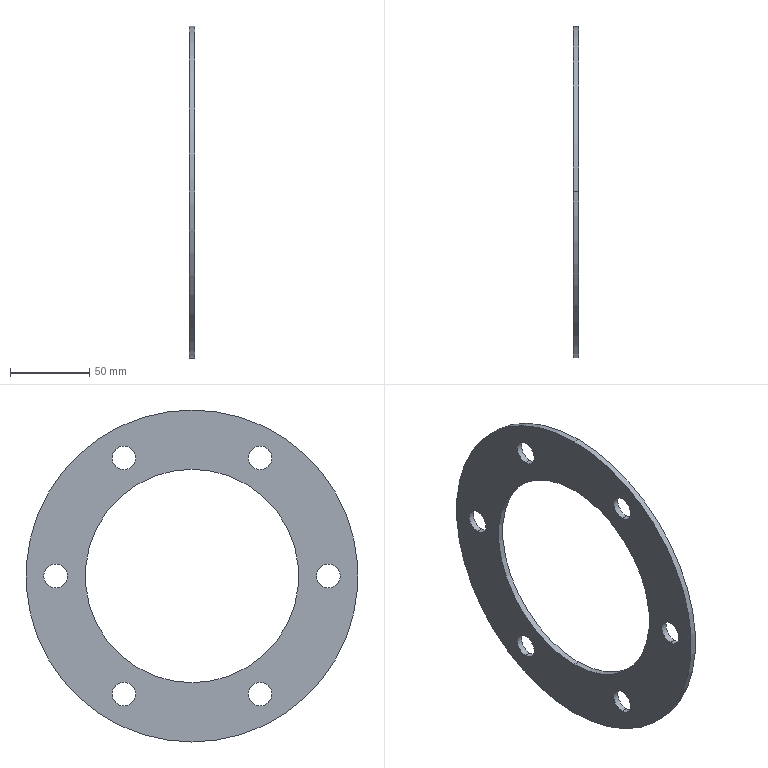Part | SolidWorks | features ICE 1, Revolution 1, Scale 1 | 1 solid | 18 faces | box 3.75 x 210 x 210 mm | volume 72232 mm3 | cylinder 16 | plane 2 | commonest cylinder face diameters 15 x12 135 x2 210 x2
STEP:
#1=CARTESIAN_POINT('',(-0.875,-43.125,67.195));
#2=VERTEX_POINT('',#1);
#3=CARTESIAN_POINT('',(-0.875,-43.125,82.195));
#4=VERTEX_POINT('',#3);
#5=CARTESIAN_POINT('',(-0.875,-43.125,74.695));
#6=DIRECTION('',(-1.,0.,0.));
#7=DIRECTION('',(0.,0.,-1.));
#8=AXIS2_PLACEMENT_3D('',#5,#6,#7);
#9=CIRCLE('',#8,7.5);
#10=EDGE_CURVE('',#2,#4,#9,.T.);
#11=ORIENTED_EDGE('',*,*,#10,.T.);
#12=CARTESIAN_POINT('',(2.875,-43.125,82.195));
#13=VERTEX_POINT('',#12);
#14=CARTESIAN_POINT('',(-15.875,-43.125,82.195));
#15=DIRECTION('',(1.,0.,0.));
#16=VECTOR('',#15,1000.);
#17=LINE('',#14,#16);
#18=EDGE_CURVE('',#4,#13,#17,.T.);
#19=ORIENTED_EDGE('',*,*,#18,.T.);
#20=CARTESIAN_POINT('',(2.875,-43.125,67.195));
#21=VERTEX_POINT('',#20);
#22=CARTESIAN_POINT('',(2.875,-43.125,74.695));
#23=DIRECTION('',(-1.,0.,0.));
#24=DIRECTION('',(0.,0.,1.));
#25=AXIS2_PLACEMENT_3D('',#22,#23,#24);
#26=CIRCLE('',#25,7.5);
#27=EDGE_CURVE('',#21,#13,#26,.T.);
#28=ORIENTED_EDGE('',*,*,#27,.F.);
#29=CARTESIAN_POINT('',(-15.875,-43.125,67.195));
#30=DIRECTION('',(1.,0.,0.));
#31=VECTOR('',#30,1000.);
#32=LINE('',#29,#31);
#33=EDGE_CURVE('',#2,#21,#32,.T.);
#34=ORIENTED_EDGE('',*,*,#33,.F.);
#35=EDGE_LOOP('',(#11,#19,#28,#34));
#36=FACE_OUTER_BOUND('',#35,.T.);
#37=CARTESIAN_POINT('',(-15.875,-43.125,74.695));
#38=DIRECTION('',(1.,0.,0.));
#39=DIRECTION('',(0.,0.,-1.));
#40=AXIS2_PLACEMENT_3D('',#37,#38,#39);
#41=CYLINDRICAL_SURFACE('',#40,7.5);
#42=ADVANCED_FACE('',(#36),#41,.F.);
#43=CARTESIAN_POINT('',(-0.875,-86.25,-7.5));
#44=VERTEX_POINT('',#43);
#45=CARTESIAN_POINT('',(-0.875,-86.25,7.5));
#46=VERTEX_POINT('',#45);
#47=CARTESIAN_POINT('',(-0.875,-86.25,0.));
#48=DIRECTION('',(-1.,0.,0.));
#49=DIRECTION('',(0.,0.,-1.));
#50=AXIS2_PLACEMENT_3D('',#47,#48,#49);
#51=CIRCLE('',#50,7.5);
#52=EDGE_CURVE('',#44,#46,#51,.T.);
#53=ORIENTED_EDGE('',*,*,#52,.T.);
#54=CARTESIAN_POINT('',(2.875,-86.25,7.5));
#55=VERTEX_POINT('',#54);
#56=CARTESIAN_POINT('',(-15.875,-86.25,7.5));
#57=DIRECTION('',(1.,0.,0.));
#58=VECTOR('',#57,1000.);
#59=LINE('',#56,#58);
#60=EDGE_CURVE('',#46,#55,#59,.T.);
#61=ORIENTED_EDGE('',*,*,#60,.T.);
#62=CARTESIAN_POINT('',(2.875,-86.25,-7.5));
#63=VERTEX_POINT('',#62);
#64=CARTESIAN_POINT('',(2.875,-86.25,0.));
#65=DIRECTION('',(-1.,0.,0.));
#66=DIRECTION('',(0.,0.,1.));
#67=AXIS2_PLACEMENT_3D('',#64,#65,#66);
#68=CIRCLE('',#67,7.5);
#69=EDGE_CURVE('',#63,#55,#68,.T.);
#70=ORIENTED_EDGE('',*,*,#69,.F.);
#71=CARTESIAN_POINT('',(-15.875,-86.25,-7.5));
#72=DIRECTION('',(1.,0.,0.));
#73=VECTOR('',#72,1000.);
#74=LINE('',#71,#73);
#75=EDGE_CURVE('',#44,#63,#74,.T.);
#76=ORIENTED_EDGE('',*,*,#75,.F.);
#77=EDGE_LOOP('',(#53,#61,#70,#76));
#78=FACE_OUTER_BOUND('',#77,.T.);
#79=CARTESIAN_POINT('',(-15.875,-86.25,0.));
#80=DIRECTION('',(1.,0.,0.));
#81=DIRECTION('',(0.,0.,-1.));
#82=AXIS2_PLACEMENT_3D('',#79,#80,#81);
#83=CYLINDRICAL_SURFACE('',#82,7.5);
#84=ADVANCED_FACE('',(#78),#83,.F.);
#85=CARTESIAN_POINT('',(-0.875,-43.125,-82.195));
#86=VERTEX_POINT('',#85);
#87=CARTESIAN_POINT('',(-0.875,-43.125,-67.195));
#88=VERTEX_POINT('',#87);
#89=CARTESIAN_POINT('',(-0.875,-43.125,-74.695));
#90=DIRECTION('',(-1.,0.,0.));
#91=DIRECTION('',(0.,0.,-1.));
#92=AXIS2_PLACEMENT_3D('',#89,#90,#91);
#93=CIRCLE('',#92,7.5);
#94=EDGE_CURVE('',#86,#88,#93,.T.);
#95=ORIENTED_EDGE('',*,*,#94,.T.);
#96=CARTESIAN_POINT('',(2.875,-43.125,-67.195));
#97=VERTEX_POINT('',#96);
#98=CARTESIAN_POINT('',(-15.875,-43.125,-67.195));
#99=DIRECTION('',(1.,0.,0.));
#100=VECTOR('',#99,1000.);
#101=LINE('',#98,#100);
#102=EDGE_CURVE('',#88,#97,#101,.T.);
#103=ORIENTED_EDGE('',*,*,#102,.T.);
#104=CARTESIAN_POINT('',(2.875,-43.125,-82.195));
#105=VERTEX_POINT('',#104);
#106=CARTESIAN_POINT('',(2.875,-43.125,-74.695));
#107=DIRECTION('',(-1.,0.,0.));
#108=DIRECTION('',(0.,0.,1.));
#109=AXIS2_PLACEMENT_3D('',#106,#107,#108);
#110=CIRCLE('',#109,7.5);
#111=EDGE_CURVE('',#105,#97,#110,.T.);
#112=ORIENTED_EDGE('',*,*,#111,.F.);
#113=CARTESIAN_POINT('',(-15.875,-43.125,-82.195));
#114=DIRECTION('',(1.,0.,0.));
#115=VECTOR('',#114,1000.);
#116=LINE('',#113,#115);
#117=EDGE_CURVE('',#86,#105,#116,.T.);
#118=ORIENTED_EDGE('',*,*,#117,.F.);
#119=EDGE_LOOP('',(#95,#103,#112,#118));
#120=FACE_OUTER_BOUND('',#119,.T.);
#121=CARTESIAN_POINT('',(-15.875,-43.125,-74.695));
#122=DIRECTION('',(1.,0.,0.));
#123=DIRECTION('',(0.,0.,-1.));
#124=AXIS2_PLACEMENT_3D('',#121,#122,#123);
#125=CYLINDRICAL_SURFACE('',#124,7.5);
#126=ADVANCED_FACE('',(#120),#125,.F.);
#127=CARTESIAN_POINT('',(-0.875,43.125,-67.195));
#128=VERTEX_POINT('',#127);
#129=CARTESIAN_POINT('',(-0.875,43.125,-82.195));
#130=VERTEX_POINT('',#129);
#131=CARTESIAN_POINT('',(-0.875,43.125,-74.695));
#132=DIRECTION('',(1.,0.,0.));
#133=DIRECTION('',(0.,0.,-1.));
#134=AXIS2_PLACEMENT_3D('',#131,#132,#133);
#135=CIRCLE('',#134,7.5);
#136=EDGE_CURVE('',#128,#130,#135,.T.);
#137=ORIENTED_EDGE('',*,*,#136,.F.);
#138=CARTESIAN_POINT('',(2.875,43.125,-67.195));
#139=VERTEX_POINT('',#138);
#140=CARTESIAN_POINT('',(-15.875,43.125,-67.195));
#141=DIRECTION('',(1.,0.,0.));
#142=VECTOR('',#141,1000.);
#143=LINE('',#140,#142);
#144=EDGE_CURVE('',#128,#139,#143,.T.);
#145=ORIENTED_EDGE('',*,*,#144,.T.);
#146=CARTESIAN_POINT('',(2.875,43.125,-82.195));
#147=VERTEX_POINT('',#146);
#148=CARTESIAN_POINT('',(2.875,43.125,-74.695));
#149=DIRECTION('',(1.,0.,0.));
#150=DIRECTION('',(0.,0.,-1.));
#151=AXIS2_PLACEMENT_3D('',#148,#149,#150);
#152=CIRCLE('',#151,7.5);
#153=EDGE_CURVE('',#139,#147,#152,.T.);
#154=ORIENTED_EDGE('',*,*,#153,.T.);
#155=CARTESIAN_POINT('',(-15.875,43.125,-82.195));
#156=DIRECTION('',(1.,0.,0.));
#157=VECTOR('',#156,1000.);
#158=LINE('',#155,#157);
#159=EDGE_CURVE('',#130,#147,#158,.T.);
#160=ORIENTED_EDGE('',*,*,#159,.F.);
#161=EDGE_LOOP('',(#137,#145,#154,#160));
#162=FACE_OUTER_BOUND('',#161,.T.);
#163=CARTESIAN_POINT('',(-15.875,43.125,-74.695));
#164=DIRECTION('',(1.,0.,0.));
#165=DIRECTION('',(0.,0.,-1.));
#166=AXIS2_PLACEMENT_3D('',#163,#164,#165);
#167=CYLINDRICAL_SURFACE('',#166,7.5);
#168=ADVANCED_FACE('',(#162),#167,.F.);
#169=CARTESIAN_POINT('',(-0.875,43.125,82.195));
#170=VERTEX_POINT('',#169);
#171=CARTESIAN_POINT('',(-0.875,43.125,67.195));
#172=VERTEX_POINT('',#171);
#173=CARTESIAN_POINT('',(-0.875,43.125,74.695));
#174=DIRECTION('',(1.,0.,0.));
#175=DIRECTION('',(0.,0.,-1.));
#176=AXIS2_PLACEMENT_3D('',#173,#174,#175);
#177=CIRCLE('',#176,7.5);
#178=EDGE_CURVE('',#170,#172,#177,.T.);
#179=ORIENTED_EDGE('',*,*,#178,.F.);
#180=CARTESIAN_POINT('',(2.875,43.125,82.195));
#181=VERTEX_POINT('',#180);
#182=CARTESIAN_POINT('',(-15.875,43.125,82.195));
#183=DIRECTION('',(1.,0.,0.));
#184=VECTOR('',#183,1000.);
#185=LINE('',#182,#184);
#186=EDGE_CURVE('',#170,#181,#185,.T.);
#187=ORIENTED_EDGE('',*,*,#186,.T.);
#188=CARTESIAN_POINT('',(2.875,43.125,67.195));
#189=VERTEX_POINT('',#188);
#190=CARTESIAN_POINT('',(2.875,43.125,74.695));
#191=DIRECTION('',(1.,0.,0.));
#192=DIRECTION('',(0.,0.,-1.));
#193=AXIS2_PLACEMENT_3D('',#190,#191,#192);
#194=CIRCLE('',#193,7.5);
#195=EDGE_CURVE('',#181,#189,#194,.T.);
#196=ORIENTED_EDGE('',*,*,#195,.T.);
#197=CARTESIAN_POINT('',(-15.875,43.125,67.195));
#198=DIRECTION('',(1.,0.,0.));
#199=VECTOR('',#198,1000.);
#200=LINE('',#197,#199);
#201=EDGE_CURVE('',#172,#189,#200,.T.);
#202=ORIENTED_EDGE('',*,*,#201,.F.);
#203=EDGE_LOOP('',(#179,#187,#196,#202));
#204=FACE_OUTER_BOUND('',#203,.T.);
#205=CARTESIAN_POINT('',(-15.875,43.125,74.695));
#206=DIRECTION('',(1.,0.,0.));
#207=DIRECTION('',(0.,0.,-1.));
#208=AXIS2_PLACEMENT_3D('',#205,#206,#207);
#209=CYLINDRICAL_SURFACE('',#208,7.5);
#210=ADVANCED_FACE('',(#204),#209,.F.);
#211=CARTESIAN_POINT('',(-0.875,86.25,7.5));
#212=VERTEX_POINT('',#211);
#213=CARTESIAN_POINT('',(-0.875,86.25,-7.5));
#214=VERTEX_POINT('',#213);
#215=CARTESIAN_POINT('',(-0.875,86.25,0.));
#216=DIRECTION('',(1.,0.,0.));
#217=DIRECTION('',(0.,0.,-1.));
#218=AXIS2_PLACEMENT_3D('',#215,#216,#217);
#219=CIRCLE('',#218,7.5);
#220=EDGE_CURVE('',#212,#214,#219,.T.);
#221=ORIENTED_EDGE('',*,*,#220,.F.);
#222=CARTESIAN_POINT('',(2.875,86.25,7.5));
#223=VERTEX_POINT('',#222);
#224=CARTESIAN_POINT('',(-15.875,86.25,7.5));
#225=DIRECTION('',(1.,0.,0.));
#226=VECTOR('',#225,1000.);
#227=LINE('',#224,#226);
#228=EDGE_CURVE('',#212,#223,#227,.T.);
#229=ORIENTED_EDGE('',*,*,#228,.T.);
#230=CARTESIAN_POINT('',(2.875,86.25,-7.5));
#231=VERTEX_POINT('',#230);
#232=CARTESIAN_POINT('',(2.875,86.25,0.));
#233=DIRECTION('',(1.,0.,0.));
#234=DIRECTION('',(0.,0.,-1.));
#235=AXIS2_PLACEMENT_3D('',#232,#233,#234);
#236=CIRCLE('',#235,7.5);
#237=EDGE_CURVE('',#223,#231,#236,.T.);
#238=ORIENTED_EDGE('',*,*,#237,.T.);
#239=CARTESIAN_POINT('',(-15.875,86.25,-7.5));
#240=DIRECTION('',(1.,0.,0.));
#241=VECTOR('',#240,1000.);
#242=LINE('',#239,#241);
#243=EDGE_CURVE('',#214,#231,#242,.T.);
#244=ORIENTED_EDGE('',*,*,#243,.F.);
#245=EDGE_LOOP('',(#221,#229,#238,#244));
#246=FACE_OUTER_BOUND('',#245,.T.);
#247=CARTESIAN_POINT('',(-15.875,86.25,0.));
#248=DIRECTION('',(1.,0.,0.));
#249=DIRECTION('',(0.,0.,-1.));
#250=AXIS2_PLACEMENT_3D('',#247,#248,#249);
#251=CYLINDRICAL_SURFACE('',#250,7.5);
#252=ADVANCED_FACE('',(#246),#251,.F.);
#253=CARTESIAN_POINT('',(2.875,0.,105.));
#254=VERTEX_POINT('',#253);
#255=CARTESIAN_POINT('',(2.875,0.,-105.));
#256=VERTEX_POINT('',#255);
#257=CARTESIAN_POINT('',(2.875,0.,0.));
#258=DIRECTION('',(-1.,0.,0.));
#259=DIRECTION('',(0.,0.,1.));
#260=AXIS2_PLACEMENT_3D('',#257,#258,#259);
#261=CIRCLE('',#260,105.);
#262=EDGE_CURVE('',#254,#256,#261,.T.);
#263=ORIENTED_EDGE('',*,*,#262,.T.);
#264=CARTESIAN_POINT('',(-0.875,0.,-105.));
#265=VERTEX_POINT('',#264);
#266=CARTESIAN_POINT('',(-0.875,0.,-105.));
#267=DIRECTION('',(-1.,0.,0.));
#268=VECTOR('',#267,1000.);
#269=LINE('',#266,#268);
#270=EDGE_CURVE('',#256,#265,#269,.T.);
#271=ORIENTED_EDGE('',*,*,#270,.T.);
#272=CARTESIAN_POINT('',(-0.875,0.,105.));
#273=VERTEX_POINT('',#272);
#274=CARTESIAN_POINT('',(-0.875,0.,0.));
#275=DIRECTION('',(-1.,0.,0.));
#276=DIRECTION('',(0.,0.,1.));
#277=AXIS2_PLACEMENT_3D('',#274,#275,#276);
#278=CIRCLE('',#277,105.);
#279=EDGE_CURVE('',#273,#265,#278,.T.);
#280=ORIENTED_EDGE('',*,*,#279,.F.);
#281=CARTESIAN_POINT('',(-0.875,0.,105.));
#282=DIRECTION('',(-1.,0.,0.));
#283=VECTOR('',#282,1000.);
#284=LINE('',#281,#283);
#285=EDGE_CURVE('',#254,#273,#284,.T.);
#286=ORIENTED_EDGE('',*,*,#285,.F.);
#287=EDGE_LOOP('',(#263,#271,#280,#286));
#288=FACE_OUTER_BOUND('',#287,.T.);
#289=CARTESIAN_POINT('',(-0.875,0.,0.));
#290=DIRECTION('',(-1.,0.,0.));
#291=DIRECTION('',(0.,0.,1.));
#292=AXIS2_PLACEMENT_3D('',#289,#290,#291);
#293=CYLINDRICAL_SURFACE('',#292,105.);
#294=ADVANCED_FACE('',(#288),#293,.T.);
#295=CARTESIAN_POINT('',(2.875,0.,-67.5));
#296=VERTEX_POINT('',#295);
#297=CARTESIAN_POINT('',(2.875,0.,67.5));
#298=VERTEX_POINT('',#297);
#299=CARTESIAN_POINT('',(2.875,0.,0.));
#300=DIRECTION('',(-1.,0.,0.));
#301=DIRECTION('',(0.,0.,1.));
#302=AXIS2_PLACEMENT_3D('',#299,#300,#301);
#303=CIRCLE('',#302,67.5);
#304=EDGE_CURVE('',#296,#298,#303,.T.);
#305=ORIENTED_EDGE('',*,*,#304,.F.);
#306=CARTESIAN_POINT('',(-0.875,0.,-67.5));
#307=VERTEX_POINT('',#306);
#308=CARTESIAN_POINT('',(-0.875,0.,-67.5));
#309=DIRECTION('',(-1.,0.,0.));
#310=VECTOR('',#309,1000.);
#311=LINE('',#308,#310);
#312=EDGE_CURVE('',#296,#307,#311,.T.);
#313=ORIENTED_EDGE('',*,*,#312,.T.);
#314=CARTESIAN_POINT('',(-0.875,0.,67.5));
#315=VERTEX_POINT('',#314);
#316=CARTESIAN_POINT('',(-0.875,0.,0.));
#317=DIRECTION('',(-1.,0.,0.));
#318=DIRECTION('',(0.,0.,1.));
#319=AXIS2_PLACEMENT_3D('',#316,#317,#318);
#320=CIRCLE('',#319,67.5);
#321=EDGE_CURVE('',#307,#315,#320,.T.);
#322=ORIENTED_EDGE('',*,*,#321,.T.);
#323=CARTESIAN_POINT('',(-0.875,0.,67.5));
#324=DIRECTION('',(-1.,0.,0.));
#325=VECTOR('',#324,1000.);
#326=LINE('',#323,#325);
#327=EDGE_CURVE('',#298,#315,#326,.T.);
#328=ORIENTED_EDGE('',*,*,#327,.F.);
#329=EDGE_LOOP('',(#305,#313,#322,#328));
#330=FACE_OUTER_BOUND('',#329,.T.);
#331=CARTESIAN_POINT('',(-0.875,0.,0.));
#332=DIRECTION('',(-1.,0.,0.));
#333=DIRECTION('',(0.,0.,1.));
#334=AXIS2_PLACEMENT_3D('',#331,#332,#333);
#335=CYLINDRICAL_SURFACE('',#334,67.5);
#336=ADVANCED_FACE('',(#330),#335,.F.);
#337=ORIENTED_EDGE('',*,*,#52,.F.);
#338=CARTESIAN_POINT('',(-0.875,-86.25,0.));
#339=DIRECTION('',(-1.,0.,0.));
#340=DIRECTION('',(0.,0.,-1.));
#341=AXIS2_PLACEMENT_3D('',#338,#339,#340);
#342=CIRCLE('',#341,7.5);
#343=EDGE_CURVE('',#46,#44,#342,.T.);
#344=ORIENTED_EDGE('',*,*,#343,.F.);
#345=EDGE_LOOP('',(#337,#344));
#346=FACE_BOUND('',#345,.T.);
#347=ORIENTED_EDGE('',*,*,#279,.T.);
#348=CARTESIAN_POINT('',(-0.875,0.,0.));
#349=DIRECTION('',(-1.,0.,0.));
#350=DIRECTION('',(0.,0.,1.));
#351=AXIS2_PLACEMENT_3D('',#348,#349,#350);
#352=CIRCLE('',#351,105.);
#353=EDGE_CURVE('',#265,#273,#352,.T.);
#354=ORIENTED_EDGE('',*,*,#353,.T.);
#355=EDGE_LOOP('',(#347,#354));
#356=FACE_OUTER_BOUND('',#355,.T.);
#357=CARTESIAN_POINT('',(-0.875,0.,0.));
#358=DIRECTION('',(-1.,0.,0.));
#359=DIRECTION('',(0.,0.,1.));
#360=AXIS2_PLACEMENT_3D('',#357,#358,#359);
#361=CIRCLE('',#360,67.5);
#362=EDGE_CURVE('',#315,#307,#361,.T.);
#363=ORIENTED_EDGE('',*,*,#362,.F.);
#364=ORIENTED_EDGE('',*,*,#321,.F.);
#365=EDGE_LOOP('',(#363,#364));
#366=FACE_BOUND('',#365,.T.);
#367=CARTESIAN_POINT('',(-0.875,86.25,0.));
#368=DIRECTION('',(1.,0.,0.));
#369=DIRECTION('',(0.,0.,-1.));
#370=AXIS2_PLACEMENT_3D('',#367,#368,#369);
#371=CIRCLE('',#370,7.5);
#372=EDGE_CURVE('',#214,#212,#371,.T.);
#373=ORIENTED_EDGE('',*,*,#372,.T.);
#374=ORIENTED_EDGE('',*,*,#220,.T.);
#375=EDGE_LOOP('',(#373,#374));
#376=FACE_BOUND('',#375,.T.);
#377=CARTESIAN_POINT('',(-0.875,43.125,74.695));
#378=DIRECTION('',(1.,0.,0.));
#379=DIRECTION('',(0.,0.,-1.));
#380=AXIS2_PLACEMENT_3D('',#377,#378,#379);
#381=CIRCLE('',#380,7.5);
#382=EDGE_CURVE('',#172,#170,#381,.T.);
#383=ORIENTED_EDGE('',*,*,#382,.T.);
#384=ORIENTED_EDGE('',*,*,#178,.T.);
#385=EDGE_LOOP('',(#383,#384));
#386=FACE_BOUND('',#385,.T.);
#387=CARTESIAN_POINT('',(-0.875,43.125,-74.695));
#388=DIRECTION('',(1.,0.,0.));
#389=DIRECTION('',(0.,0.,-1.));
#390=AXIS2_PLACEMENT_3D('',#387,#388,#389);
#391=CIRCLE('',#390,7.5);
#392=EDGE_CURVE('',#130,#128,#391,.T.);
#393=ORIENTED_EDGE('',*,*,#392,.T.);
#394=ORIENTED_EDGE('',*,*,#136,.T.);
#395=EDGE_LOOP('',(#393,#394));
#396=FACE_BOUND('',#395,.T.);
#397=ORIENTED_EDGE('',*,*,#94,.F.);
#398=CARTESIAN_POINT('',(-0.875,-43.125,-74.695));
#399=DIRECTION('',(-1.,0.,0.));
#400=DIRECTION('',(0.,0.,-1.));
#401=AXIS2_PLACEMENT_3D('',#398,#399,#400);
#402=CIRCLE('',#401,7.5);
#403=EDGE_CURVE('',#88,#86,#402,.T.);
#404=ORIENTED_EDGE('',*,*,#403,.F.);
#405=EDGE_LOOP('',(#397,#404));
#406=FACE_BOUND('',#405,.T.);
#407=ORIENTED_EDGE('',*,*,#10,.F.);
#408=CARTESIAN_POINT('',(-0.875,-43.125,74.695));
#409=DIRECTION('',(-1.,0.,0.));
#410=DIRECTION('',(0.,0.,-1.));
#411=AXIS2_PLACEMENT_3D('',#408,#409,#410);
#412=CIRCLE('',#411,7.5);
#413=EDGE_CURVE('',#4,#2,#412,.T.);
#414=ORIENTED_EDGE('',*,*,#413,.F.);
#415=EDGE_LOOP('',(#407,#414));
#416=FACE_BOUND('',#415,.T.);
#417=CARTESIAN_POINT('',(-0.875,105.,0.));
#418=DIRECTION('',(1.,0.,0.));
#419=DIRECTION('',(0.,0.,-1.));
#420=AXIS2_PLACEMENT_3D('',#417,#418,#419);
#421=PLANE('',#420);
#422=ADVANCED_FACE('',(#346,#356,#366,#376,#386,#396,#406,#416),#421,.F.);
#423=ORIENTED_EDGE('',*,*,#69,.T.);
#424=CARTESIAN_POINT('',(2.875,-86.25,0.));
#425=DIRECTION('',(-1.,0.,0.));
#426=DIRECTION('',(0.,0.,1.));
#427=AXIS2_PLACEMENT_3D('',#424,#425,#426);
#428=CIRCLE('',#427,7.5);
#429=EDGE_CURVE('',#55,#63,#428,.T.);
#430=ORIENTED_EDGE('',*,*,#429,.T.);
#431=EDGE_LOOP('',(#423,#430));
#432=FACE_BOUND('',#431,.T.);
#433=CARTESIAN_POINT('',(2.875,0.,0.));
#434=DIRECTION('',(-1.,0.,0.));
#435=DIRECTION('',(0.,0.,1.));
#436=AXIS2_PLACEMENT_3D('',#433,#434,#435);
#437=CIRCLE('',#436,67.5);
#438=EDGE_CURVE('',#298,#296,#437,.T.);
#439=ORIENTED_EDGE('',*,*,#438,.T.);
#440=ORIENTED_EDGE('',*,*,#304,.T.);
#441=EDGE_LOOP('',(#439,#440));
#442=FACE_BOUND('',#441,.T.);
#443=ORIENTED_EDGE('',*,*,#262,.F.);
#444=CARTESIAN_POINT('',(2.875,0.,0.));
#445=DIRECTION('',(-1.,0.,0.));
#446=DIRECTION('',(0.,0.,1.));
#447=AXIS2_PLACEMENT_3D('',#444,#445,#446);
#448=CIRCLE('',#447,105.);
#449=EDGE_CURVE('',#256,#254,#448,.T.);
#450=ORIENTED_EDGE('',*,*,#449,.F.);
#451=EDGE_LOOP('',(#443,#450));
#452=FACE_OUTER_BOUND('',#451,.T.);
#453=CARTESIAN_POINT('',(2.875,86.25,0.));
#454=DIRECTION('',(1.,0.,0.));
#455=DIRECTION('',(0.,0.,-1.));
#456=AXIS2_PLACEMENT_3D('',#453,#454,#455);
#457=CIRCLE('',#456,7.5);
#458=EDGE_CURVE('',#231,#223,#457,.T.);
#459=ORIENTED_EDGE('',*,*,#458,.F.);
#460=ORIENTED_EDGE('',*,*,#237,.F.);
#461=EDGE_LOOP('',(#459,#460));
#462=FACE_BOUND('',#461,.T.);
#463=CARTESIAN_POINT('',(2.875,43.125,74.695));
#464=DIRECTION('',(1.,0.,0.));
#465=DIRECTION('',(0.,0.,-1.));
#466=AXIS2_PLACEMENT_3D('',#463,#464,#465);
#467=CIRCLE('',#466,7.5);
#468=EDGE_CURVE('',#189,#181,#467,.T.);
#469=ORIENTED_EDGE('',*,*,#468,.F.);
#470=ORIENTED_EDGE('',*,*,#195,.F.);
#471=EDGE_LOOP('',(#469,#470));
#472=FACE_BOUND('',#471,.T.);
#473=CARTESIAN_POINT('',(2.875,43.125,-74.695));
#474=DIRECTION('',(1.,0.,0.));
#475=DIRECTION('',(0.,0.,-1.));
#476=AXIS2_PLACEMENT_3D('',#473,#474,#475);
#477=CIRCLE('',#476,7.5);
#478=EDGE_CURVE('',#147,#139,#477,.T.);
#479=ORIENTED_EDGE('',*,*,#478,.F.);
#480=ORIENTED_EDGE('',*,*,#153,.F.);
#481=EDGE_LOOP('',(#479,#480));
#482=FACE_BOUND('',#481,.T.);
#483=ORIENTED_EDGE('',*,*,#111,.T.);
#484=CARTESIAN_POINT('',(2.875,-43.125,-74.695));
#485=DIRECTION('',(-1.,0.,0.));
#486=DIRECTION('',(0.,0.,1.));
#487=AXIS2_PLACEMENT_3D('',#484,#485,#486);
#488=CIRCLE('',#487,7.5);
#489=EDGE_CURVE('',#97,#105,#488,.T.);
#490=ORIENTED_EDGE('',*,*,#489,.T.);
#491=EDGE_LOOP('',(#483,#490));
#492=FACE_BOUND('',#491,.T.);
#493=ORIENTED_EDGE('',*,*,#27,.T.);
#494=CARTESIAN_POINT('',(2.875,-43.125,74.695));
#495=DIRECTION('',(-1.,0.,0.));
#496=DIRECTION('',(0.,0.,1.));
#497=AXIS2_PLACEMENT_3D('',#494,#495,#496);
#498=CIRCLE('',#497,7.5);
#499=EDGE_CURVE('',#13,#21,#498,.T.);
#500=ORIENTED_EDGE('',*,*,#499,.T.);
#501=EDGE_LOOP('',(#493,#500));
#502=FACE_BOUND('',#501,.T.);
#503=CARTESIAN_POINT('',(2.875,105.,0.));
#504=DIRECTION('',(-1.,0.,0.));
#505=DIRECTION('',(0.,0.,1.));
#506=AXIS2_PLACEMENT_3D('',#503,#504,#505);
#507=PLANE('',#506);
#508=ADVANCED_FACE('',(#432,#442,#452,#462,#472,#482,#492,#502),#507,.F.);
#509=ORIENTED_EDGE('',*,*,#312,.F.);
#510=ORIENTED_EDGE('',*,*,#438,.F.);
#511=ORIENTED_EDGE('',*,*,#327,.T.);
#512=ORIENTED_EDGE('',*,*,#362,.T.);
#513=EDGE_LOOP('',(#509,#510,#511,#512));
#514=FACE_OUTER_BOUND('',#513,.T.);
#515=CARTESIAN_POINT('',(-0.875,0.,0.));
#516=DIRECTION('',(-1.,0.,0.));
#517=DIRECTION('',(0.,0.,1.));
#518=AXIS2_PLACEMENT_3D('',#515,#516,#517);
#519=CYLINDRICAL_SURFACE('',#518,67.5);
#520=ADVANCED_FACE('',(#514),#519,.F.);
#521=ORIENTED_EDGE('',*,*,#270,.F.);
#522=ORIENTED_EDGE('',*,*,#449,.T.);
#523=ORIENTED_EDGE('',*,*,#285,.T.);
#524=ORIENTED_EDGE('',*,*,#353,.F.);
#525=EDGE_LOOP('',(#521,#522,#523,#524));
#526=FACE_OUTER_BOUND('',#525,.T.);
#527=CARTESIAN_POINT('',(-0.875,0.,0.));
#528=DIRECTION('',(-1.,0.,0.));
#529=DIRECTION('',(0.,0.,1.));
#530=AXIS2_PLACEMENT_3D('',#527,#528,#529);
#531=CYLINDRICAL_SURFACE('',#530,105.);
#532=ADVANCED_FACE('',(#526),#531,.T.);
#533=ORIENTED_EDGE('',*,*,#228,.F.);
#534=ORIENTED_EDGE('',*,*,#372,.F.);
#535=ORIENTED_EDGE('',*,*,#243,.T.);
#536=ORIENTED_EDGE('',*,*,#458,.T.);
#537=EDGE_LOOP('',(#533,#534,#535,#536));
#538=FACE_OUTER_BOUND('',#537,.T.);
#539=CARTESIAN_POINT('',(-15.875,86.25,0.));
#540=DIRECTION('',(1.,0.,0.));
#541=DIRECTION('',(0.,0.,-1.));
#542=AXIS2_PLACEMENT_3D('',#539,#540,#541);
#543=CYLINDRICAL_SURFACE('',#542,7.5);
#544=ADVANCED_FACE('',(#538),#543,.F.);
#545=ORIENTED_EDGE('',*,*,#186,.F.);
#546=ORIENTED_EDGE('',*,*,#382,.F.);
#547=ORIENTED_EDGE('',*,*,#201,.T.);
#548=ORIENTED_EDGE('',*,*,#468,.T.);
#549=EDGE_LOOP('',(#545,#546,#547,#548));
#550=FACE_OUTER_BOUND('',#549,.T.);
#551=CARTESIAN_POINT('',(-15.875,43.125,74.695));
#552=DIRECTION('',(1.,0.,0.));
#553=DIRECTION('',(0.,0.,-1.));
#554=AXIS2_PLACEMENT_3D('',#551,#552,#553);
#555=CYLINDRICAL_SURFACE('',#554,7.5);
#556=ADVANCED_FACE('',(#550),#555,.F.);
#557=ORIENTED_EDGE('',*,*,#144,.F.);
#558=ORIENTED_EDGE('',*,*,#392,.F.);
#559=ORIENTED_EDGE('',*,*,#159,.T.);
#560=ORIENTED_EDGE('',*,*,#478,.T.);
#561=EDGE_LOOP('',(#557,#558,#559,#560));
#562=FACE_OUTER_BOUND('',#561,.T.);
#563=CARTESIAN_POINT('',(-15.875,43.125,-74.695));
#564=DIRECTION('',(1.,0.,0.));
#565=DIRECTION('',(0.,0.,-1.));
#566=AXIS2_PLACEMENT_3D('',#563,#564,#565);
#567=CYLINDRICAL_SURFACE('',#566,7.5);
#568=ADVANCED_FACE('',(#562),#567,.F.);
#569=ORIENTED_EDGE('',*,*,#102,.F.);
#570=ORIENTED_EDGE('',*,*,#403,.T.);
#571=ORIENTED_EDGE('',*,*,#117,.T.);
#572=ORIENTED_EDGE('',*,*,#489,.F.);
#573=EDGE_LOOP('',(#569,#570,#571,#572));
#574=FACE_OUTER_BOUND('',#573,.T.);
#575=CARTESIAN_POINT('',(-15.875,-43.125,-74.695));
#576=DIRECTION('',(1.,0.,0.));
#577=DIRECTION('',(0.,0.,-1.));
#578=AXIS2_PLACEMENT_3D('',#575,#576,#577);
#579=CYLINDRICAL_SURFACE('',#578,7.5);
#580=ADVANCED_FACE('',(#574),#579,.F.);
#581=ORIENTED_EDGE('',*,*,#60,.F.);
#582=ORIENTED_EDGE('',*,*,#343,.T.);
#583=ORIENTED_EDGE('',*,*,#75,.T.);
#584=ORIENTED_EDGE('',*,*,#429,.F.);
#585=EDGE_LOOP('',(#581,#582,#583,#584));
#586=FACE_OUTER_BOUND('',#585,.T.);
#587=CARTESIAN_POINT('',(-15.875,-86.25,0.));
#588=DIRECTION('',(1.,0.,0.));
#589=DIRECTION('',(0.,0.,-1.));
#590=AXIS2_PLACEMENT_3D('',#587,#588,#589);
#591=CYLINDRICAL_SURFACE('',#590,7.5);
#592=ADVANCED_FACE('',(#586),#591,.F.);
#593=ORIENTED_EDGE('',*,*,#18,.F.);
#594=ORIENTED_EDGE('',*,*,#413,.T.);
#595=ORIENTED_EDGE('',*,*,#33,.T.);
#596=ORIENTED_EDGE('',*,*,#499,.F.);
#597=EDGE_LOOP('',(#593,#594,#595,#596));
#598=FACE_OUTER_BOUND('',#597,.T.);
#599=CARTESIAN_POINT('',(-15.875,-43.125,74.695));
#600=DIRECTION('',(1.,0.,0.));
#601=DIRECTION('',(0.,0.,-1.));
#602=AXIS2_PLACEMENT_3D('',#599,#600,#601);
#603=CYLINDRICAL_SURFACE('',#602,7.5);
#604=ADVANCED_FACE('',(#598),#603,.F.);
#605=CLOSED_SHELL('',(#42,#84,#126,#168,#210,#252,#294,#336,#422,#508,#520,#532,#544,#556,#568,#580,#592,#604));
#606=MANIFOLD_SOLID_BREP('',#605);
#607=CARTESIAN_POINT('',(0.,0.,0.));
#608=DIRECTION('',(0.,0.,1.));
#609=DIRECTION('',(1.,0.,0.));
#610=AXIS2_PLACEMENT_3D('',#607,#608,#609);
#611=(LENGTH_UNIT()NAMED_UNIT(*)SI_UNIT(.MILLI.,.METRE.));
#612=UNCERTAINTY_MEASURE_WITH_UNIT(LENGTH_MEASURE(0.00001),#611,'','');
#613=(NAMED_UNIT(*)PLANE_ANGLE_UNIT()SI_UNIT($,.RADIAN.));
#614=(NAMED_UNIT(*)SI_UNIT($,.STERADIAN.)SOLID_ANGLE_UNIT());
#615=(GEOMETRIC_REPRESENTATION_CONTEXT(3)GLOBAL_UNCERTAINTY_ASSIGNED_CONTEXT((#612))GLOBAL_UNIT_ASSIGNED_CONTEXT((#611,#613,#614))REPRESENTATION_CONTEXT('',''));
#616=ADVANCED_BREP_SHAPE_REPRESENTATION('',(#606,#610),#615);